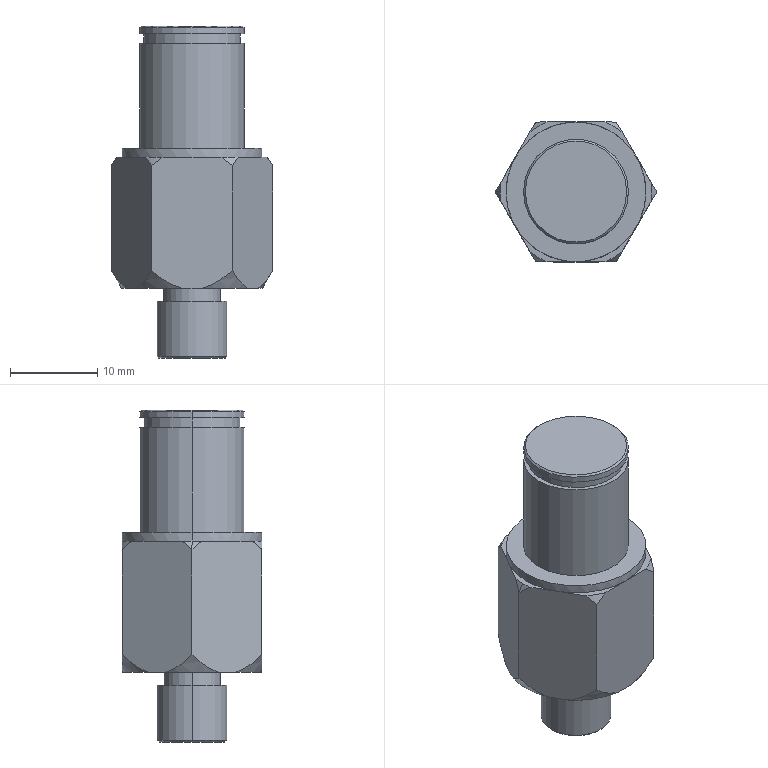Part | SolidWorks | features Cut 3, ICE 3, Chamfer 1, Extrusion 1, RevCut 1 | 1 solid | 49 faces | box 18.475 x 16 x 38 mm | volume 5453 mm3 | plane 19 | cone 18 | cylinder 12 | commonest cylinder face diameters 12 x4 6.5 x2 8 x2 11 x2 16 x2
STEP:
#1=CARTESIAN_POINT('',(-8.587,48.872,15.));
#2=VERTEX_POINT('',#1);
#3=CARTESIAN_POINT('',(-8.66,50.,15.));
#4=VERTEX_POINT('',#3);
#5=CARTESIAN_POINT('',(0.,50.,15.));
#6=DIRECTION('',(0.,0.,-1.));
#7=DIRECTION('',(-1.,0.,0.));
#8=AXIS2_PLACEMENT_3D('',#5,#6,#7);
#9=CIRCLE('',#8,8.66);
#10=EDGE_CURVE('',#2,#4,#9,.T.);
#11=ORIENTED_EDGE('',*,*,#10,.T.);
#12=CARTESIAN_POINT('',(-9.238,50.,14.));
#13=VERTEX_POINT('',#12);
#14=CARTESIAN_POINT('',(-8.66,50.,15.));
#15=DIRECTION('',(-0.5,0.,-0.866));
#16=VECTOR('',#15,1000.);
#17=LINE('',#14,#16);
#18=EDGE_CURVE('',#4,#13,#17,.T.);
#19=ORIENTED_EDGE('',*,*,#18,.T.);
#20=CARTESIAN_POINT('',(-9.238,50.,14.));
#21=CARTESIAN_POINT('',(-9.03,49.641,14.359));
#22=CARTESIAN_POINT('',(-8.815,49.268,14.697));
#23=CARTESIAN_POINT('',(-8.587,48.872,15.));
#24=B_SPLINE_CURVE_WITH_KNOTS('',3,(#20,#21,#22,#23),.UNSPECIFIED.,.F.,.F.,(4,4),(0.007442,0.009078),.UNSPECIFIED.);
#25=EDGE_CURVE('',#13,#2,#24,.T.);
#26=ORIENTED_EDGE('',*,*,#25,.T.);
#27=EDGE_LOOP('',(#11,#19,#26));
#28=FACE_OUTER_BOUND('',#27,.T.);
#29=CARTESIAN_POINT('',(0.,50.,15.));
#30=DIRECTION('',(0.,0.,-1.));
#31=DIRECTION('',(-1.,0.,0.));
#32=AXIS2_PLACEMENT_3D('',#29,#30,#31);
#33=CONICAL_SURFACE('',#32,8.66,0.5236);
#34=ADVANCED_FACE('',(#28),#33,.T.);
#35=CARTESIAN_POINT('',(8.083,50.,0.));
#36=VERTEX_POINT('',#35);
#37=CARTESIAN_POINT('',(7.506,47.,0.));
#38=VERTEX_POINT('',#37);
#39=CARTESIAN_POINT('',(0.,50.,0.));
#40=DIRECTION('',(0.,0.,-1.));
#41=DIRECTION('',(-1.,0.,0.));
#42=AXIS2_PLACEMENT_3D('',#39,#40,#41);
#43=CIRCLE('',#42,8.083);
#44=EDGE_CURVE('',#36,#38,#43,.T.);
#45=ORIENTED_EDGE('',*,*,#44,.F.);
#46=CARTESIAN_POINT('',(9.238,50.,2.));
#47=VERTEX_POINT('',#46);
#48=CARTESIAN_POINT('',(9.238,50.,2.));
#49=DIRECTION('',(0.5,0.,0.866));
#50=VECTOR('',#49,1000.);
#51=LINE('',#48,#50);
#52=EDGE_CURVE('',#36,#47,#51,.T.);
#53=ORIENTED_EDGE('',*,*,#52,.T.);
#54=CARTESIAN_POINT('',(9.238,50.,2.));
#55=CARTESIAN_POINT('',(8.982,49.558,1.558));
#56=CARTESIAN_POINT('',(8.714,49.094,1.146));
#57=CARTESIAN_POINT('',(8.136,48.093,0.4442));
#58=CARTESIAN_POINT('',(7.833,47.568,0.1622));
#59=CARTESIAN_POINT('',(7.506,47.,0.));
#60=B_SPLINE_CURVE_WITH_KNOTS('',3,(#54,#55,#56,#57,#58,#59),.UNSPECIFIED.,.F.,.F.,(4,2,4),(0.007563,0.009578,0.01159),.UNSPECIFIED.);
#61=EDGE_CURVE('',#47,#38,#60,.T.);
#62=ORIENTED_EDGE('',*,*,#61,.T.);
#63=EDGE_LOOP('',(#45,#53,#62));
#64=FACE_OUTER_BOUND('',#63,.T.);
#65=CARTESIAN_POINT('',(0.,50.,2.));
#66=DIRECTION('',(0.,0.,1.));
#67=DIRECTION('',(1.,0.,0.));
#68=AXIS2_PLACEMENT_3D('',#65,#66,#67);
#69=CONICAL_SURFACE('',#68,9.238,0.5236);
#70=ADVANCED_FACE('',(#64),#69,.T.);
#71=CARTESIAN_POINT('',(5.8,50.,30.));
#72=VERTEX_POINT('',#71);
#73=CARTESIAN_POINT('',(-5.8,50.,30.));
#74=VERTEX_POINT('',#73);
#75=CARTESIAN_POINT('',(0.,50.,30.));
#76=DIRECTION('',(0.,0.,1.));
#77=DIRECTION('',(1.,0.,0.));
#78=AXIS2_PLACEMENT_3D('',#75,#76,#77);
#79=CIRCLE('',#78,5.8);
#80=EDGE_CURVE('',#72,#74,#79,.T.);
#81=ORIENTED_EDGE('',*,*,#80,.F.);
#82=CARTESIAN_POINT('',(6.,50.,29.8));
#83=VERTEX_POINT('',#82);
#84=CARTESIAN_POINT('',(5.8,50.,30.));
#85=DIRECTION('',(0.7071,0.,-0.7071));
#86=VECTOR('',#85,1000.);
#87=LINE('',#84,#86);
#88=EDGE_CURVE('',#72,#83,#87,.T.);
#89=ORIENTED_EDGE('',*,*,#88,.T.);
#90=CARTESIAN_POINT('',(-6.,50.,29.8));
#91=VERTEX_POINT('',#90);
#92=CARTESIAN_POINT('',(0.,50.,29.8));
#93=DIRECTION('',(0.,0.,-1.));
#94=DIRECTION('',(1.,0.,0.));
#95=AXIS2_PLACEMENT_3D('',#92,#93,#94);
#96=CIRCLE('',#95,6.);
#97=EDGE_CURVE('',#91,#83,#96,.T.);
#98=ORIENTED_EDGE('',*,*,#97,.F.);
#99=CARTESIAN_POINT('',(-5.8,50.,30.));
#100=DIRECTION('',(-0.7071,0.,-0.7071));
#101=VECTOR('',#100,1000.);
#102=LINE('',#99,#101);
#103=EDGE_CURVE('',#74,#91,#102,.T.);
#104=ORIENTED_EDGE('',*,*,#103,.F.);
#105=EDGE_LOOP('',(#81,#89,#98,#104));
#106=FACE_OUTER_BOUND('',#105,.T.);
#107=CARTESIAN_POINT('',(0.,50.,30.));
#108=DIRECTION('',(0.,0.,-1.));
#109=DIRECTION('',(-1.,0.,0.));
#110=AXIS2_PLACEMENT_3D('',#107,#108,#109);
#111=CONICAL_SURFACE('',#110,5.8,0.7854);
#112=ADVANCED_FACE('',(#106),#111,.T.);
#113=CARTESIAN_POINT('',(-3.8,50.,-8.));
#114=VERTEX_POINT('',#113);
#115=CARTESIAN_POINT('',(3.8,50.,-8.));
#116=VERTEX_POINT('',#115);
#117=CARTESIAN_POINT('',(0.,50.,-8.));
#118=DIRECTION('',(0.,0.,-1.));
#119=DIRECTION('',(-1.,0.,0.));
#120=AXIS2_PLACEMENT_3D('',#117,#118,#119);
#121=CIRCLE('',#120,3.8);
#122=EDGE_CURVE('',#114,#116,#121,.T.);
#123=ORIENTED_EDGE('',*,*,#122,.F.);
#124=CARTESIAN_POINT('',(-4.,50.,-7.8));
#125=VERTEX_POINT('',#124);
#126=CARTESIAN_POINT('',(-3.8,50.,-8.));
#127=DIRECTION('',(-0.7071,0.,0.7071));
#128=VECTOR('',#127,1000.);
#129=LINE('',#126,#128);
#130=EDGE_CURVE('',#114,#125,#129,.T.);
#131=ORIENTED_EDGE('',*,*,#130,.T.);
#132=CARTESIAN_POINT('',(4.,50.,-7.8));
#133=VERTEX_POINT('',#132);
#134=CARTESIAN_POINT('',(0.,50.,-7.8));
#135=DIRECTION('',(0.,0.,1.));
#136=DIRECTION('',(-1.,0.,0.));
#137=AXIS2_PLACEMENT_3D('',#134,#135,#136);
#138=CIRCLE('',#137,4.);
#139=EDGE_CURVE('',#133,#125,#138,.T.);
#140=ORIENTED_EDGE('',*,*,#139,.F.);
#141=CARTESIAN_POINT('',(3.8,50.,-8.));
#142=DIRECTION('',(0.7071,0.,0.7071));
#143=VECTOR('',#142,1000.);
#144=LINE('',#141,#143);
#145=EDGE_CURVE('',#116,#133,#144,.T.);
#146=ORIENTED_EDGE('',*,*,#145,.F.);
#147=EDGE_LOOP('',(#123,#131,#140,#146));
#148=FACE_OUTER_BOUND('',#147,.T.);
#149=CARTESIAN_POINT('',(0.,50.,-8.));
#150=DIRECTION('',(0.,0.,1.));
#151=DIRECTION('',(1.,0.,0.));
#152=AXIS2_PLACEMENT_3D('',#149,#150,#151);
#153=CONICAL_SURFACE('',#152,3.8,0.7854);
#154=ADVANCED_FACE('',(#148),#153,.T.);
#155=CARTESIAN_POINT('',(-6.,50.,29.1));
#156=VERTEX_POINT('',#155);
#157=CARTESIAN_POINT('',(6.,50.,29.1));
#158=VERTEX_POINT('',#157);
#159=CARTESIAN_POINT('',(0.,50.,29.1));
#160=DIRECTION('',(0.,0.,-1.));
#161=DIRECTION('',(1.,0.,0.));
#162=AXIS2_PLACEMENT_3D('',#159,#160,#161);
#163=CIRCLE('',#162,6.);
#164=EDGE_CURVE('',#156,#158,#163,.T.);
#165=ORIENTED_EDGE('',*,*,#164,.F.);
#166=CARTESIAN_POINT('',(-6.,50.,16.));
#167=DIRECTION('',(0.,0.,1.));
#168=VECTOR('',#167,1000.);
#169=LINE('',#166,#168);
#170=EDGE_CURVE('',#156,#91,#169,.T.);
#171=ORIENTED_EDGE('',*,*,#170,.T.);
#172=ORIENTED_EDGE('',*,*,#97,.T.);
#173=CARTESIAN_POINT('',(6.,50.,16.));
#174=DIRECTION('',(0.,0.,1.));
#175=VECTOR('',#174,1000.);
#176=LINE('',#173,#175);
#177=EDGE_CURVE('',#158,#83,#176,.T.);
#178=ORIENTED_EDGE('',*,*,#177,.F.);
#179=EDGE_LOOP('',(#165,#171,#172,#178));
#180=FACE_OUTER_BOUND('',#179,.T.);
#181=CARTESIAN_POINT('',(0.,50.,16.));
#182=DIRECTION('',(0.,0.,1.));
#183=DIRECTION('',(1.,0.,0.));
#184=AXIS2_PLACEMENT_3D('',#181,#182,#183);
#185=CYLINDRICAL_SURFACE('',#184,6.);
#186=ADVANCED_FACE('',(#180),#185,.T.);
#187=CARTESIAN_POINT('',(5.5,50.,29.1));
#188=VERTEX_POINT('',#187);
#189=CARTESIAN_POINT('',(-5.5,50.,29.1));
#190=VERTEX_POINT('',#189);
#191=CARTESIAN_POINT('',(0.,50.,29.1));
#192=DIRECTION('',(0.,0.,1.));
#193=DIRECTION('',(1.,0.,0.));
#194=AXIS2_PLACEMENT_3D('',#191,#192,#193);
#195=CIRCLE('',#194,5.5);
#196=EDGE_CURVE('',#188,#190,#195,.T.);
#197=ORIENTED_EDGE('',*,*,#196,.F.);
#198=CARTESIAN_POINT('',(5.5,50.,28.));
#199=VERTEX_POINT('',#198);
#200=CARTESIAN_POINT('',(5.5,50.,29.1));
#201=DIRECTION('',(0.,0.,-1.));
#202=VECTOR('',#201,1000.);
#203=LINE('',#200,#202);
#204=EDGE_CURVE('',#188,#199,#203,.T.);
#205=ORIENTED_EDGE('',*,*,#204,.T.);
#206=CARTESIAN_POINT('',(-5.5,50.,28.));
#207=VERTEX_POINT('',#206);
#208=CARTESIAN_POINT('',(0.,50.,28.));
#209=DIRECTION('',(0.,0.,1.));
#210=DIRECTION('',(1.,0.,0.));
#211=AXIS2_PLACEMENT_3D('',#208,#209,#210);
#212=CIRCLE('',#211,5.5);
#213=EDGE_CURVE('',#199,#207,#212,.T.);
#214=ORIENTED_EDGE('',*,*,#213,.T.);
#215=CARTESIAN_POINT('',(-5.5,50.,29.1));
#216=DIRECTION('',(0.,0.,-1.));
#217=VECTOR('',#216,1000.);
#218=LINE('',#215,#217);
#219=EDGE_CURVE('',#190,#207,#218,.T.);
#220=ORIENTED_EDGE('',*,*,#219,.F.);
#221=EDGE_LOOP('',(#197,#205,#214,#220));
#222=FACE_OUTER_BOUND('',#221,.T.);
#223=CARTESIAN_POINT('',(0.,50.,29.1));
#224=DIRECTION('',(0.,0.,-1.));
#225=DIRECTION('',(-1.,0.,0.));
#226=AXIS2_PLACEMENT_3D('',#223,#224,#225);
#227=CYLINDRICAL_SURFACE('',#226,5.5);
#228=ADVANCED_FACE('',(#222),#227,.T.);
#229=ORIENTED_EDGE('',*,*,#139,.T.);
#230=CARTESIAN_POINT('',(-4.,50.,-1.5));
#231=VERTEX_POINT('',#230);
#232=CARTESIAN_POINT('',(-4.,50.,-8.));
#233=DIRECTION('',(0.,0.,1.));
#234=VECTOR('',#233,1000.);
#235=LINE('',#232,#234);
#236=EDGE_CURVE('',#125,#231,#235,.T.);
#237=ORIENTED_EDGE('',*,*,#236,.T.);
#238=CARTESIAN_POINT('',(4.,50.,-1.5));
#239=VERTEX_POINT('',#238);
#240=CARTESIAN_POINT('',(0.,50.,-1.5));
#241=DIRECTION('',(0.,0.,-1.));
#242=DIRECTION('',(-1.,0.,0.));
#243=AXIS2_PLACEMENT_3D('',#240,#241,#242);
#244=CIRCLE('',#243,4.);
#245=EDGE_CURVE('',#231,#239,#244,.T.);
#246=ORIENTED_EDGE('',*,*,#245,.T.);
#247=CARTESIAN_POINT('',(4.,50.,-8.));
#248=DIRECTION('',(0.,0.,1.));
#249=VECTOR('',#248,1000.);
#250=LINE('',#247,#249);
#251=EDGE_CURVE('',#133,#239,#250,.T.);
#252=ORIENTED_EDGE('',*,*,#251,.F.);
#253=EDGE_LOOP('',(#229,#237,#246,#252));
#254=FACE_OUTER_BOUND('',#253,.T.);
#255=CARTESIAN_POINT('',(0.,50.,-8.));
#256=DIRECTION('',(0.,0.,1.));
#257=DIRECTION('',(1.,0.,0.));
#258=AXIS2_PLACEMENT_3D('',#255,#256,#257);
#259=CYLINDRICAL_SURFACE('',#258,4.);
#260=ADVANCED_FACE('',(#254),#259,.T.);
#261=CARTESIAN_POINT('',(-3.25,50.,-1.5));
#262=VERTEX_POINT('',#261);
#263=CARTESIAN_POINT('',(3.25,50.,-1.5));
#264=VERTEX_POINT('',#263);
#265=CARTESIAN_POINT('',(0.,50.,-1.5));
#266=DIRECTION('',(0.,0.,-1.));
#267=DIRECTION('',(-1.,0.,0.));
#268=AXIS2_PLACEMENT_3D('',#265,#266,#267);
#269=CIRCLE('',#268,3.25);
#270=EDGE_CURVE('',#262,#264,#269,.T.);
#271=ORIENTED_EDGE('',*,*,#270,.F.);
#272=CARTESIAN_POINT('',(-3.25,50.,0.));
#273=VERTEX_POINT('',#272);
#274=CARTESIAN_POINT('',(-3.25,50.,-1.5));
#275=DIRECTION('',(0.,0.,1.));
#276=VECTOR('',#275,1000.);
#277=LINE('',#274,#276);
#278=EDGE_CURVE('',#262,#273,#277,.T.);
#279=ORIENTED_EDGE('',*,*,#278,.T.);
#280=CARTESIAN_POINT('',(3.25,50.,0.));
#281=VERTEX_POINT('',#280);
#282=CARTESIAN_POINT('',(0.,50.,0.));
#283=DIRECTION('',(0.,0.,-1.));
#284=DIRECTION('',(-1.,0.,0.));
#285=AXIS2_PLACEMENT_3D('',#282,#283,#284);
#286=CIRCLE('',#285,3.25);
#287=EDGE_CURVE('',#273,#281,#286,.T.);
#288=ORIENTED_EDGE('',*,*,#287,.T.);
#289=CARTESIAN_POINT('',(3.25,50.,-1.5));
#290=DIRECTION('',(0.,0.,1.));
#291=VECTOR('',#290,1000.);
#292=LINE('',#289,#291);
#293=EDGE_CURVE('',#264,#281,#292,.T.);
#294=ORIENTED_EDGE('',*,*,#293,.F.);
#295=EDGE_LOOP('',(#271,#279,#288,#294));
#296=FACE_OUTER_BOUND('',#295,.T.);
#297=CARTESIAN_POINT('',(0.,50.,-1.5));
#298=DIRECTION('',(0.,0.,1.));
#299=DIRECTION('',(1.,0.,0.));
#300=AXIS2_PLACEMENT_3D('',#297,#298,#299);
#301=CYLINDRICAL_SURFACE('',#300,3.25);
#302=ADVANCED_FACE('',(#296),#301,.T.);
#303=CARTESIAN_POINT('',(-8.,50.,16.));
#304=VERTEX_POINT('',#303);
#305=CARTESIAN_POINT('',(8.,50.,16.));
#306=VERTEX_POINT('',#305);
#307=CARTESIAN_POINT('',(0.,50.,16.));
#308=DIRECTION('',(0.,0.,-1.));
#309=DIRECTION('',(1.,0.,0.));
#310=AXIS2_PLACEMENT_3D('',#307,#308,#309);
#311=CIRCLE('',#310,8.);
#312=EDGE_CURVE('',#304,#306,#311,.T.);
#313=ORIENTED_EDGE('',*,*,#312,.T.);
#314=CARTESIAN_POINT('',(8.,50.,15.));
#315=VERTEX_POINT('',#314);
#316=CARTESIAN_POINT('',(8.,50.,30.));
#317=DIRECTION('',(0.,0.,-1.));
#318=VECTOR('',#317,1000.);
#319=LINE('',#316,#318);
#320=EDGE_CURVE('',#306,#315,#319,.T.);
#321=ORIENTED_EDGE('',*,*,#320,.T.);
#322=CARTESIAN_POINT('',(6.928,54.,15.));
#323=VERTEX_POINT('',#322);
#324=CARTESIAN_POINT('',(0.,50.,15.));
#325=DIRECTION('',(0.,0.,-1.));
#326=DIRECTION('',(-1.,0.,0.));
#327=AXIS2_PLACEMENT_3D('',#324,#325,#326);
#328=CIRCLE('',#327,8.);
#329=EDGE_CURVE('',#323,#315,#328,.T.);
#330=ORIENTED_EDGE('',*,*,#329,.F.);
#331=CARTESIAN_POINT('',(0.,58.,15.));
#332=VERTEX_POINT('',#331);
#333=CARTESIAN_POINT('',(0.,50.,15.));
#334=DIRECTION('',(0.,0.,-1.));
#335=DIRECTION('',(-1.,0.,0.));
#336=AXIS2_PLACEMENT_3D('',#333,#334,#335);
#337=CIRCLE('',#336,8.);
#338=EDGE_CURVE('',#332,#323,#337,.T.);
#339=ORIENTED_EDGE('',*,*,#338,.F.);
#340=CARTESIAN_POINT('',(-6.928,54.,15.));
#341=VERTEX_POINT('',#340);
#342=CARTESIAN_POINT('',(0.,50.,15.));
#343=DIRECTION('',(0.,0.,-1.));
#344=DIRECTION('',(-1.,0.,0.));
#345=AXIS2_PLACEMENT_3D('',#342,#343,#344);
#346=CIRCLE('',#345,8.);
#347=EDGE_CURVE('',#341,#332,#346,.T.);
#348=ORIENTED_EDGE('',*,*,#347,.F.);
#349=CARTESIAN_POINT('',(-8.,50.,15.));
#350=VERTEX_POINT('',#349);
#351=CARTESIAN_POINT('',(0.,50.,15.));
#352=DIRECTION('',(0.,0.,-1.));
#353=DIRECTION('',(-1.,0.,0.));
#354=AXIS2_PLACEMENT_3D('',#351,#352,#353);
#355=CIRCLE('',#354,8.);
#356=EDGE_CURVE('',#350,#341,#355,.T.);
#357=ORIENTED_EDGE('',*,*,#356,.F.);
#358=CARTESIAN_POINT('',(-8.,50.,30.));
#359=DIRECTION('',(0.,0.,-1.));
#360=VECTOR('',#359,1000.);
#361=LINE('',#358,#360);
#362=EDGE_CURVE('',#304,#350,#361,.T.);
#363=ORIENTED_EDGE('',*,*,#362,.F.);
#364=EDGE_LOOP('',(#313,#321,#330,#339,#348,#357,#363));
#365=FACE_OUTER_BOUND('',#364,.T.);
#366=CARTESIAN_POINT('',(0.,50.,30.));
#367=DIRECTION('',(0.,0.,-1.));
#368=DIRECTION('',(-1.,0.,0.));
#369=AXIS2_PLACEMENT_3D('',#366,#367,#368);
#370=CYLINDRICAL_SURFACE('',#369,8.);
#371=ADVANCED_FACE('',(#365),#370,.T.);
#372=CARTESIAN_POINT('',(6.,50.,16.));
#373=VERTEX_POINT('',#372);
#374=CARTESIAN_POINT('',(-6.,50.,16.));
#375=VERTEX_POINT('',#374);
#376=CARTESIAN_POINT('',(0.,50.,16.));
#377=DIRECTION('',(0.,0.,1.));
#378=DIRECTION('',(1.,0.,0.));
#379=AXIS2_PLACEMENT_3D('',#376,#377,#378);
#380=CIRCLE('',#379,6.);
#381=EDGE_CURVE('',#373,#375,#380,.T.);
#382=ORIENTED_EDGE('',*,*,#381,.T.);
#383=CARTESIAN_POINT('',(-6.,50.,28.));
#384=VERTEX_POINT('',#383);
#385=CARTESIAN_POINT('',(-6.,50.,16.));
#386=DIRECTION('',(0.,0.,1.));
#387=VECTOR('',#386,1000.);
#388=LINE('',#385,#387);
#389=EDGE_CURVE('',#375,#384,#388,.T.);
#390=ORIENTED_EDGE('',*,*,#389,.T.);
#391=CARTESIAN_POINT('',(6.,50.,28.));
#392=VERTEX_POINT('',#391);
#393=CARTESIAN_POINT('',(0.,50.,28.));
#394=DIRECTION('',(0.,0.,-1.));
#395=DIRECTION('',(1.,0.,0.));
#396=AXIS2_PLACEMENT_3D('',#393,#394,#395);
#397=CIRCLE('',#396,6.);
#398=EDGE_CURVE('',#384,#392,#397,.T.);
#399=ORIENTED_EDGE('',*,*,#398,.T.);
#400=CARTESIAN_POINT('',(6.,50.,16.));
#401=DIRECTION('',(0.,0.,1.));
#402=VECTOR('',#401,1000.);
#403=LINE('',#400,#402);
#404=EDGE_CURVE('',#373,#392,#403,.T.);
#405=ORIENTED_EDGE('',*,*,#404,.F.);
#406=EDGE_LOOP('',(#382,#390,#399,#405));
#407=FACE_OUTER_BOUND('',#406,.T.);
#408=CARTESIAN_POINT('',(0.,50.,16.));
#409=DIRECTION('',(0.,0.,1.));
#410=DIRECTION('',(1.,0.,0.));
#411=AXIS2_PLACEMENT_3D('',#408,#409,#410);
#412=CYLINDRICAL_SURFACE('',#411,6.);
#413=ADVANCED_FACE('',(#407),#412,.T.);
#414=ORIENTED_EDGE('',*,*,#389,.F.);
#415=CARTESIAN_POINT('',(0.,50.,16.));
#416=DIRECTION('',(0.,0.,1.));
#417=DIRECTION('',(1.,0.,0.));
#418=AXIS2_PLACEMENT_3D('',#415,#416,#417);
#419=CIRCLE('',#418,6.);
#420=EDGE_CURVE('',#375,#373,#419,.T.);
#421=ORIENTED_EDGE('',*,*,#420,.T.);
#422=ORIENTED_EDGE('',*,*,#404,.T.);
#423=CARTESIAN_POINT('',(0.,50.,28.));
#424=DIRECTION('',(0.,0.,-1.));
#425=DIRECTION('',(1.,0.,0.));
#426=AXIS2_PLACEMENT_3D('',#423,#424,#425);
#427=CIRCLE('',#426,6.);
#428=EDGE_CURVE('',#392,#384,#427,.T.);
#429=ORIENTED_EDGE('',*,*,#428,.T.);
#430=EDGE_LOOP('',(#414,#421,#422,#429));
#431=FACE_OUTER_BOUND('',#430,.T.);
#432=CARTESIAN_POINT('',(0.,50.,16.));
#433=DIRECTION('',(0.,0.,1.));
#434=DIRECTION('',(1.,0.,0.));
#435=AXIS2_PLACEMENT_3D('',#432,#433,#434);
#436=CYLINDRICAL_SURFACE('',#435,6.);
#437=ADVANCED_FACE('',(#431),#436,.T.);
#438=ORIENTED_EDGE('',*,*,#320,.F.);
#439=CARTESIAN_POINT('',(0.,50.,16.));
#440=DIRECTION('',(0.,0.,-1.));
#441=DIRECTION('',(1.,0.,0.));
#442=AXIS2_PLACEMENT_3D('',#439,#440,#441);
#443=CIRCLE('',#442,8.);
#444=EDGE_CURVE('',#306,#304,#443,.T.);
#445=ORIENTED_EDGE('',*,*,#444,.T.);
#446=ORIENTED_EDGE('',*,*,#362,.T.);
#447=CARTESIAN_POINT('',(-6.928,46.,15.));
#448=VERTEX_POINT('',#447);
#449=CARTESIAN_POINT('',(0.,50.,15.));
#450=DIRECTION('',(0.,0.,-1.));
#451=DIRECTION('',(-1.,0.,0.));
#452=AXIS2_PLACEMENT_3D('',#449,#450,#451);
#453=CIRCLE('',#452,8.);
#454=EDGE_CURVE('',#448,#350,#453,.T.);
#455=ORIENTED_EDGE('',*,*,#454,.F.);
#456=CARTESIAN_POINT('',(0.,42.,15.));
#457=VERTEX_POINT('',#456);
#458=CARTESIAN_POINT('',(0.,50.,15.));
#459=DIRECTION('',(0.,0.,-1.));
#460=DIRECTION('',(-1.,0.,0.));
#461=AXIS2_PLACEMENT_3D('',#458,#459,#460);
#462=CIRCLE('',#461,8.);
#463=EDGE_CURVE('',#457,#448,#462,.T.);
#464=ORIENTED_EDGE('',*,*,#463,.F.);
#465=CARTESIAN_POINT('',(6.928,46.,15.));
#466=VERTEX_POINT('',#465);
#467=CARTESIAN_POINT('',(0.,50.,15.));
#468=DIRECTION('',(0.,0.,-1.));
#469=DIRECTION('',(-1.,0.,0.));
#470=AXIS2_PLACEMENT_3D('',#467,#468,#469);
#471=CIRCLE('',#470,8.);
#472=EDGE_CURVE('',#466,#457,#471,.T.);
#473=ORIENTED_EDGE('',*,*,#472,.F.);
#474=CARTESIAN_POINT('',(0.,50.,15.));
#475=DIRECTION('',(0.,0.,-1.));
#476=DIRECTION('',(-1.,0.,0.));
#477=AXIS2_PLACEMENT_3D('',#474,#475,#476);
#478=CIRCLE('',#477,8.);
#479=EDGE_CURVE('',#315,#466,#478,.T.);
#480=ORIENTED_EDGE('',*,*,#479,.F.);
#481=EDGE_LOOP('',(#438,#445,#446,#455,#464,#473,#480));
#482=FACE_OUTER_BOUND('',#481,.T.);
#483=CARTESIAN_POINT('',(0.,50.,30.));
#484=DIRECTION('',(0.,0.,-1.));
#485=DIRECTION('',(-1.,0.,0.));
#486=AXIS2_PLACEMENT_3D('',#483,#484,#485);
#487=CYLINDRICAL_SURFACE('',#486,8.);
#488=ADVANCED_FACE('',(#482),#487,.T.);
#489=CARTESIAN_POINT('',(6.351,45.,0.));
#490=VERTEX_POINT('',#489);
#491=CARTESIAN_POINT('',(9.238,50.,0.));
#492=DIRECTION('',(-0.5,-0.866,0.));
#493=VECTOR('',#492,1000.);
#494=LINE('',#491,#493);
#495=EDGE_CURVE('',#38,#490,#494,.T.);
#496=ORIENTED_EDGE('',*,*,#495,.T.);
#497=CARTESIAN_POINT('',(1.155,42.,0.));
#498=VERTEX_POINT('',#497);
#499=CARTESIAN_POINT('',(0.,50.,0.));
#500=DIRECTION('',(0.,0.,-1.));
#501=DIRECTION('',(-1.,0.,0.));
#502=AXIS2_PLACEMENT_3D('',#499,#500,#501);
#503=CIRCLE('',#502,8.083);
#504=EDGE_CURVE('',#490,#498,#503,.T.);
#505=ORIENTED_EDGE('',*,*,#504,.T.);
#506=CARTESIAN_POINT('',(-1.155,42.,0.));
#507=VERTEX_POINT('',#506);
#508=CARTESIAN_POINT('',(4.619,42.,0.));
#509=DIRECTION('',(-1.,0.,0.));
#510=VECTOR('',#509,1000.);
#511=LINE('',#508,#510);
#512=EDGE_CURVE('',#498,#507,#511,.T.);
#513=ORIENTED_EDGE('',*,*,#512,.T.);
#514=CARTESIAN_POINT('',(-6.351,45.,0.));
#515=VERTEX_POINT('',#514);
#516=CARTESIAN_POINT('',(0.,50.,0.));
#517=DIRECTION('',(0.,0.,-1.));
#518=DIRECTION('',(-1.,0.,0.));
#519=AXIS2_PLACEMENT_3D('',#516,#517,#518);
#520=CIRCLE('',#519,8.083);
#521=EDGE_CURVE('',#507,#515,#520,.T.);
#522=ORIENTED_EDGE('',*,*,#521,.T.);
#523=CARTESIAN_POINT('',(-7.506,47.,0.));
#524=VERTEX_POINT('',#523);
#525=CARTESIAN_POINT('',(-4.619,42.,0.));
#526=DIRECTION('',(-0.5,0.866,0.));
#527=VECTOR('',#526,1000.);
#528=LINE('',#525,#527);
#529=EDGE_CURVE('',#515,#524,#528,.T.);
#530=ORIENTED_EDGE('',*,*,#529,.T.);
#531=CARTESIAN_POINT('',(-7.506,53.,0.));
#532=VERTEX_POINT('',#531);
#533=CARTESIAN_POINT('',(0.,50.,0.));
#534=DIRECTION('',(0.,0.,-1.));
#535=DIRECTION('',(-1.,0.,0.));
#536=AXIS2_PLACEMENT_3D('',#533,#534,#535);
#537=CIRCLE('',#536,8.083);
#538=EDGE_CURVE('',#524,#532,#537,.T.);
#539=ORIENTED_EDGE('',*,*,#538,.T.);
#540=CARTESIAN_POINT('',(-6.351,55.,0.));
#541=VERTEX_POINT('',#540);
#542=CARTESIAN_POINT('',(-9.238,50.,0.));
#543=DIRECTION('',(0.5,0.866,0.));
#544=VECTOR('',#543,1000.);
#545=LINE('',#542,#544);
#546=EDGE_CURVE('',#532,#541,#545,.T.);
#547=ORIENTED_EDGE('',*,*,#546,.T.);
#548=CARTESIAN_POINT('',(-1.155,58.,0.));
#549=VERTEX_POINT('',#548);
#550=CARTESIAN_POINT('',(0.,50.,0.));
#551=DIRECTION('',(0.,0.,-1.));
#552=DIRECTION('',(-1.,0.,0.));
#553=AXIS2_PLACEMENT_3D('',#550,#551,#552);
#554=CIRCLE('',#553,8.083);
#555=EDGE_CURVE('',#541,#549,#554,.T.);
#556=ORIENTED_EDGE('',*,*,#555,.T.);
#557=CARTESIAN_POINT('',(1.155,58.,0.));
#558=VERTEX_POINT('',#557);
#559=CARTESIAN_POINT('',(-4.619,58.,0.));
#560=DIRECTION('',(1.,0.,0.));
#561=VECTOR('',#560,1000.);
#562=LINE('',#559,#561);
#563=EDGE_CURVE('',#549,#558,#562,.T.);
#564=ORIENTED_EDGE('',*,*,#563,.T.);
#565=CARTESIAN_POINT('',(6.351,55.,0.));
#566=VERTEX_POINT('',#565);
#567=CARTESIAN_POINT('',(0.,50.,0.));
#568=DIRECTION('',(0.,0.,-1.));
#569=DIRECTION('',(-1.,0.,0.));
#570=AXIS2_PLACEMENT_3D('',#567,#568,#569);
#571=CIRCLE('',#570,8.083);
#572=EDGE_CURVE('',#558,#566,#571,.T.);
#573=ORIENTED_EDGE('',*,*,#572,.T.);
#574=CARTESIAN_POINT('',(7.506,53.,0.));
#575=VERTEX_POINT('',#574);
#576=CARTESIAN_POINT('',(4.619,58.,0.));
#577=DIRECTION('',(0.5,-0.866,0.));
#578=VECTOR('',#577,1000.);
#579=LINE('',#576,#578);
#580=EDGE_CURVE('',#566,#575,#579,.T.);
#581=ORIENTED_EDGE('',*,*,#580,.T.);
#582=CARTESIAN_POINT('',(0.,50.,0.));
#583=DIRECTION('',(0.,0.,-1.));
#584=DIRECTION('',(-1.,0.,0.));
#585=AXIS2_PLACEMENT_3D('',#582,#583,#584);
#586=CIRCLE('',#585,8.083);
#587=EDGE_CURVE('',#575,#36,#586,.T.);
#588=ORIENTED_EDGE('',*,*,#587,.T.);
#589=ORIENTED_EDGE('',*,*,#44,.T.);
#590=EDGE_LOOP('',(#496,#505,#513,#522,#530,#539,#547,#556,#564,#573,#581,#588,#589));
#591=FACE_OUTER_BOUND('',#590,.T.);
#592=CARTESIAN_POINT('',(0.,50.,0.));
#593=DIRECTION('',(0.,0.,-1.));
#594=DIRECTION('',(-1.,0.,0.));
#595=AXIS2_PLACEMENT_3D('',#592,#593,#594);
#596=CIRCLE('',#595,3.25);
#597=EDGE_CURVE('',#281,#273,#596,.T.);
#598=ORIENTED_EDGE('',*,*,#597,.F.);
#599=ORIENTED_EDGE('',*,*,#287,.F.);
#600=EDGE_LOOP('',(#598,#599));
#601=FACE_BOUND('',#600,.T.);
#602=CARTESIAN_POINT('',(0.,50.,0.));
#603=DIRECTION('',(0.,0.,1.));
#604=DIRECTION('',(1.,0.,0.));
#605=AXIS2_PLACEMENT_3D('',#602,#603,#604);
#606=PLANE('',#605);
#607=ADVANCED_FACE('',(#591,#601),#606,.F.);
#608=CARTESIAN_POINT('',(-4.619,42.,14.));
#609=VERTEX_POINT('',#608);
#610=CARTESIAN_POINT('',(-3.317,42.,15.));
#611=VERTEX_POINT('',#610);
#612=CARTESIAN_POINT('',(-4.619,42.,14.));
#613=CARTESIAN_POINT('',(-4.204,42.,14.359));
#614=CARTESIAN_POINT('',(-3.773,42.,14.697));
#615=CARTESIAN_POINT('',(-3.317,42.,15.));
#616=B_SPLINE_CURVE_WITH_KNOTS('',3,(#612,#613,#614,#615),.UNSPECIFIED.,.F.,.F.,(4,4),(0.007442,0.009078),.UNSPECIFIED.);
#617=EDGE_CURVE('',#609,#611,#616,.T.);
#618=ORIENTED_EDGE('',*,*,#617,.F.);
#619=CARTESIAN_POINT('',(-4.619,42.,2.));
#620=VERTEX_POINT('',#619);
#621=CARTESIAN_POINT('',(-4.619,42.,15.));
#622=DIRECTION('',(0.,0.,-1.));
#623=VECTOR('',#622,1000.);
#624=LINE('',#621,#623);
#625=EDGE_CURVE('',#609,#620,#624,.T.);
#626=ORIENTED_EDGE('',*,*,#625,.T.);
#627=CARTESIAN_POINT('',(-1.155,42.,0.));
#628=CARTESIAN_POINT('',(-1.482,42.,0.08107));
#629=CARTESIAN_POINT('',(-1.8,42.,0.1933));
#630=CARTESIAN_POINT('',(-2.419,42.,0.4666));
#631=CARTESIAN_POINT('',(-2.718,42.,0.627));
#632=CARTESIAN_POINT('',(-3.578,42.,1.151));
#633=CARTESIAN_POINT('',(-4.11,42.,1.559));
#634=CARTESIAN_POINT('',(-4.619,42.,2.));
#635=B_SPLINE_CURVE_WITH_KNOTS('',3,(#627,#628,#629,#630,#631,#632,#633,#634),.UNSPECIFIED.,.F.,.F.,(4,2,2,4),(0.01391,0.01491,0.01592,0.01793),.UNSPECIFIED.);
#636=EDGE_CURVE('',#507,#620,#635,.T.);
#637=ORIENTED_EDGE('',*,*,#636,.F.);
#638=ORIENTED_EDGE('',*,*,#512,.F.);
#639=CARTESIAN_POINT('',(4.619,42.,2.));
#640=VERTEX_POINT('',#639);
#641=CARTESIAN_POINT('',(4.619,42.,2.));
#642=CARTESIAN_POINT('',(4.109,42.,1.558));
#643=CARTESIAN_POINT('',(3.572,42.,1.146));
#644=CARTESIAN_POINT('',(2.416,42.,0.4442));
#645=CARTESIAN_POINT('',(1.81,42.,0.1622));
#646=CARTESIAN_POINT('',(1.155,42.,0.));
#647=B_SPLINE_CURVE_WITH_KNOTS('',3,(#641,#642,#643,#644,#645,#646),.UNSPECIFIED.,.F.,.F.,(4,2,4),(0.007563,0.009578,0.01159),.UNSPECIFIED.);
#648=EDGE_CURVE('',#640,#498,#647,.T.);
#649=ORIENTED_EDGE('',*,*,#648,.F.);
#650=CARTESIAN_POINT('',(4.619,42.,14.));
#651=VERTEX_POINT('',#650);
#652=CARTESIAN_POINT('',(4.619,42.,15.));
#653=DIRECTION('',(0.,0.,-1.));
#654=VECTOR('',#653,1000.);
#655=LINE('',#652,#654);
#656=EDGE_CURVE('',#651,#640,#655,.T.);
#657=ORIENTED_EDGE('',*,*,#656,.F.);
#658=CARTESIAN_POINT('',(3.317,42.,15.));
#659=VERTEX_POINT('',#658);
#660=CARTESIAN_POINT('',(3.317,42.,15.));
#661=CARTESIAN_POINT('',(3.772,42.,14.698));
#662=CARTESIAN_POINT('',(4.203,42.,14.36));
#663=CARTESIAN_POINT('',(4.619,42.,14.));
#664=B_SPLINE_CURVE_WITH_KNOTS('',3,(#660,#661,#662,#663),.UNSPECIFIED.,.F.,.F.,(4,4),(0.01616,0.0178),.UNSPECIFIED.);
#665=EDGE_CURVE('',#659,#651,#664,.T.);
#666=ORIENTED_EDGE('',*,*,#665,.F.);
#667=CARTESIAN_POINT('',(4.619,42.,15.));
#668=DIRECTION('',(-1.,0.,0.));
#669=VECTOR('',#668,1000.);
#670=LINE('',#667,#669);
#671=EDGE_CURVE('',#659,#457,#670,.T.);
#672=ORIENTED_EDGE('',*,*,#671,.T.);
#673=CARTESIAN_POINT('',(4.619,42.,15.));
#674=DIRECTION('',(-1.,0.,0.));
#675=VECTOR('',#674,1000.);
#676=LINE('',#673,#675);
#677=EDGE_CURVE('',#457,#611,#676,.T.);
#678=ORIENTED_EDGE('',*,*,#677,.T.);
#679=EDGE_LOOP('',(#618,#626,#637,#638,#649,#657,#666,#672,#678));
#680=FACE_OUTER_BOUND('',#679,.T.);
#681=CARTESIAN_POINT('',(4.619,42.,15.));
#682=DIRECTION('',(0.,-1.,0.));
#683=DIRECTION('',(0.,0.,-1.));
#684=AXIS2_PLACEMENT_3D('',#681,#682,#683);
#685=PLANE('',#684);
#686=ADVANCED_FACE('',(#680),#685,.T.);
#687=ORIENTED_EDGE('',*,*,#25,.F.);
#688=CARTESIAN_POINT('',(-9.238,50.,2.));
#689=VERTEX_POINT('',#688);
#690=CARTESIAN_POINT('',(-9.238,50.,15.));
#691=DIRECTION('',(0.,0.,-1.));
#692=VECTOR('',#691,1000.);
#693=LINE('',#690,#692);
#694=EDGE_CURVE('',#13,#689,#693,.T.);
#695=ORIENTED_EDGE('',*,*,#694,.T.);
#696=CARTESIAN_POINT('',(-7.506,47.,0.));
#697=CARTESIAN_POINT('',(-7.669,47.284,0.08107));
#698=CARTESIAN_POINT('',(-7.828,47.559,0.1933));
#699=CARTESIAN_POINT('',(-8.138,48.095,0.4666));
#700=CARTESIAN_POINT('',(-8.287,48.354,0.627));
#701=CARTESIAN_POINT('',(-8.717,49.099,1.151));
#702=CARTESIAN_POINT('',(-8.983,49.559,1.559));
#703=CARTESIAN_POINT('',(-9.238,50.,2.));
#704=B_SPLINE_CURVE_WITH_KNOTS('',3,(#696,#697,#698,#699,#700,#701,#702,#703),.UNSPECIFIED.,.F.,.F.,(4,2,2,4),(0.01391,0.01491,0.01592,0.01793),.UNSPECIFIED.);
#705=EDGE_CURVE('',#524,#689,#704,.T.);
#706=ORIENTED_EDGE('',*,*,#705,.F.);
#707=ORIENTED_EDGE('',*,*,#529,.F.);
#708=CARTESIAN_POINT('',(-4.619,42.,2.));
#709=CARTESIAN_POINT('',(-4.874,42.442,1.558));
#710=CARTESIAN_POINT('',(-5.142,42.906,1.146));
#711=CARTESIAN_POINT('',(-5.72,43.907,0.4442));
#712=CARTESIAN_POINT('',(-6.023,44.432,0.1622));
#713=CARTESIAN_POINT('',(-6.351,45.,0.));
#714=B_SPLINE_CURVE_WITH_KNOTS('',3,(#708,#709,#710,#711,#712,#713),.UNSPECIFIED.,.F.,.F.,(4,2,4),(0.007563,0.009578,0.01159),.UNSPECIFIED.);
#715=EDGE_CURVE('',#620,#515,#714,.T.);
#716=ORIENTED_EDGE('',*,*,#715,.F.);
#717=ORIENTED_EDGE('',*,*,#625,.F.);
#718=CARTESIAN_POINT('',(-5.27,43.128,15.));
#719=VERTEX_POINT('',#718);
#720=CARTESIAN_POINT('',(-5.27,43.128,15.));
#721=CARTESIAN_POINT('',(-5.042,42.734,14.698));
#722=CARTESIAN_POINT('',(-4.827,42.36,14.36));
#723=CARTESIAN_POINT('',(-4.619,42.,14.));
#724=B_SPLINE_CURVE_WITH_KNOTS('',3,(#720,#721,#722,#723),.UNSPECIFIED.,.F.,.F.,(4,4),(0.01616,0.0178),.UNSPECIFIED.);
#725=EDGE_CURVE('',#719,#609,#724,.T.);
#726=ORIENTED_EDGE('',*,*,#725,.F.);
#727=CARTESIAN_POINT('',(-4.619,42.,15.));
#728=DIRECTION('',(-0.5,0.866,0.));
#729=VECTOR('',#728,1000.);
#730=LINE('',#727,#729);
#731=EDGE_CURVE('',#719,#448,#730,.T.);
#732=ORIENTED_EDGE('',*,*,#731,.T.);
#733=CARTESIAN_POINT('',(-4.619,42.,15.));
#734=DIRECTION('',(0.5,-0.866,0.));
#735=VECTOR('',#734,1000.);
#736=LINE('',#733,#735);
#737=EDGE_CURVE('',#2,#448,#736,.T.);
#738=ORIENTED_EDGE('',*,*,#737,.F.);
#739=EDGE_LOOP('',(#687,#695,#706,#707,#716,#717,#726,#732,#738));
#740=FACE_OUTER_BOUND('',#739,.T.);
#741=CARTESIAN_POINT('',(-4.619,42.,15.));
#742=DIRECTION('',(-0.866,-0.5,0.));
#743=DIRECTION('',(0.5,-0.866,0.));
#744=AXIS2_PLACEMENT_3D('',#741,#742,#743);
#745=PLANE('',#744);
#746=ADVANCED_FACE('',(#740),#745,.T.);
#747=CARTESIAN_POINT('',(-4.619,58.,14.));
#748=VERTEX_POINT('',#747);
#749=CARTESIAN_POINT('',(-5.27,56.872,15.));
#750=VERTEX_POINT('',#749);
#751=CARTESIAN_POINT('',(-4.619,58.,14.));
#752=CARTESIAN_POINT('',(-4.826,57.641,14.359));
#753=CARTESIAN_POINT('',(-5.042,57.268,14.697));
#754=CARTESIAN_POINT('',(-5.27,56.872,15.));
#755=B_SPLINE_CURVE_WITH_KNOTS('',3,(#751,#752,#753,#754),.UNSPECIFIED.,.F.,.F.,(4,4),(0.007442,0.009078),.UNSPECIFIED.);
#756=EDGE_CURVE('',#748,#750,#755,.T.);
#757=ORIENTED_EDGE('',*,*,#756,.F.);
#758=CARTESIAN_POINT('',(-4.619,58.,2.));
#759=VERTEX_POINT('',#758);
#760=CARTESIAN_POINT('',(-4.619,58.,15.));
#761=DIRECTION('',(0.,0.,-1.));
#762=VECTOR('',#761,1000.);
#763=LINE('',#760,#762);
#764=EDGE_CURVE('',#748,#759,#763,.T.);
#765=ORIENTED_EDGE('',*,*,#764,.T.);
#766=CARTESIAN_POINT('',(-6.351,55.,0.));
#767=CARTESIAN_POINT('',(-6.187,55.284,0.08107));
#768=CARTESIAN_POINT('',(-6.028,55.559,0.1933));
#769=CARTESIAN_POINT('',(-5.719,56.095,0.4666));
#770=CARTESIAN_POINT('',(-5.569,56.354,0.627));
#771=CARTESIAN_POINT('',(-5.139,57.099,1.151));
#772=CARTESIAN_POINT('',(-4.873,57.559,1.559));
#773=CARTESIAN_POINT('',(-4.619,58.,2.));
#774=B_SPLINE_CURVE_WITH_KNOTS('',3,(#766,#767,#768,#769,#770,#771,#772,#773),.UNSPECIFIED.,.F.,.F.,(4,2,2,4),(0.01391,0.01491,0.01592,0.01793),.UNSPECIFIED.);
#775=EDGE_CURVE('',#541,#759,#774,.T.);
#776=ORIENTED_EDGE('',*,*,#775,.F.);
#777=ORIENTED_EDGE('',*,*,#546,.F.);
#778=CARTESIAN_POINT('',(-9.238,50.,2.));
#779=CARTESIAN_POINT('',(-8.982,50.442,1.558));
#780=CARTESIAN_POINT('',(-8.714,50.906,1.146));
#781=CARTESIAN_POINT('',(-8.136,51.907,0.4442));
#782=CARTESIAN_POINT('',(-7.833,52.432,0.1622));
#783=CARTESIAN_POINT('',(-7.506,53.,0.));
#784=B_SPLINE_CURVE_WITH_KNOTS('',3,(#778,#779,#780,#781,#782,#783),.UNSPECIFIED.,.F.,.F.,(4,2,4),(0.007563,0.009578,0.01159),.UNSPECIFIED.);
#785=EDGE_CURVE('',#689,#532,#784,.T.);
#786=ORIENTED_EDGE('',*,*,#785,.F.);
#787=ORIENTED_EDGE('',*,*,#694,.F.);
#788=CARTESIAN_POINT('',(-8.587,51.128,15.));
#789=VERTEX_POINT('',#788);
#790=CARTESIAN_POINT('',(-8.587,51.128,15.));
#791=CARTESIAN_POINT('',(-8.814,50.734,14.698));
#792=CARTESIAN_POINT('',(-9.03,50.36,14.36));
#793=CARTESIAN_POINT('',(-9.238,50.,14.));
#794=B_SPLINE_CURVE_WITH_KNOTS('',3,(#790,#791,#792,#793),.UNSPECIFIED.,.F.,.F.,(4,4),(0.01616,0.0178),.UNSPECIFIED.);
#795=EDGE_CURVE('',#789,#13,#794,.T.);
#796=ORIENTED_EDGE('',*,*,#795,.F.);
#797=CARTESIAN_POINT('',(-9.238,50.,15.));
#798=DIRECTION('',(0.5,0.866,0.));
#799=VECTOR('',#798,1000.);
#800=LINE('',#797,#799);
#801=EDGE_CURVE('',#789,#341,#800,.T.);
#802=ORIENTED_EDGE('',*,*,#801,.T.);
#803=CARTESIAN_POINT('',(-9.238,50.,15.));
#804=DIRECTION('',(-0.5,-0.866,0.));
#805=VECTOR('',#804,1000.);
#806=LINE('',#803,#805);
#807=EDGE_CURVE('',#750,#341,#806,.T.);
#808=ORIENTED_EDGE('',*,*,#807,.F.);
#809=EDGE_LOOP('',(#757,#765,#776,#777,#786,#787,#796,#802,#808));
#810=FACE_OUTER_BOUND('',#809,.T.);
#811=CARTESIAN_POINT('',(-9.238,50.,15.));
#812=DIRECTION('',(-0.866,0.5,0.));
#813=DIRECTION('',(-0.5,-0.866,0.));
#814=AXIS2_PLACEMENT_3D('',#811,#812,#813);
#815=PLANE('',#814);
#816=ADVANCED_FACE('',(#810),#815,.T.);
#817=CARTESIAN_POINT('',(4.619,58.,14.));
#818=VERTEX_POINT('',#817);
#819=CARTESIAN_POINT('',(3.317,58.,15.));
#820=VERTEX_POINT('',#819);
#821=CARTESIAN_POINT('',(4.619,58.,14.));
#822=CARTESIAN_POINT('',(4.204,58.,14.359));
#823=CARTESIAN_POINT('',(3.773,58.,14.697));
#824=CARTESIAN_POINT('',(3.317,58.,15.));
#825=B_SPLINE_CURVE_WITH_KNOTS('',3,(#821,#822,#823,#824),.UNSPECIFIED.,.F.,.F.,(4,4),(0.007442,0.009078),.UNSPECIFIED.);
#826=EDGE_CURVE('',#818,#820,#825,.T.);
#827=ORIENTED_EDGE('',*,*,#826,.F.);
#828=CARTESIAN_POINT('',(4.619,58.,2.));
#829=VERTEX_POINT('',#828);
#830=CARTESIAN_POINT('',(4.619,58.,15.));
#831=DIRECTION('',(0.,0.,-1.));
#832=VECTOR('',#831,1000.);
#833=LINE('',#830,#832);
#834=EDGE_CURVE('',#818,#829,#833,.T.);
#835=ORIENTED_EDGE('',*,*,#834,.T.);
#836=CARTESIAN_POINT('',(1.155,58.,0.));
#837=CARTESIAN_POINT('',(1.482,58.,0.08107));
#838=CARTESIAN_POINT('',(1.8,58.,0.1933));
#839=CARTESIAN_POINT('',(2.419,58.,0.4666));
#840=CARTESIAN_POINT('',(2.718,58.,0.627));
#841=CARTESIAN_POINT('',(3.578,58.,1.151));
#842=CARTESIAN_POINT('',(4.11,58.,1.559));
#843=CARTESIAN_POINT('',(4.619,58.,2.));
#844=B_SPLINE_CURVE_WITH_KNOTS('',3,(#836,#837,#838,#839,#840,#841,#842,#843),.UNSPECIFIED.,.F.,.F.,(4,2,2,4),(0.01391,0.01491,0.01592,0.01793),.UNSPECIFIED.);
#845=EDGE_CURVE('',#558,#829,#844,.T.);
#846=ORIENTED_EDGE('',*,*,#845,.F.);
#847=ORIENTED_EDGE('',*,*,#563,.F.);
#848=CARTESIAN_POINT('',(-4.619,58.,2.));
#849=CARTESIAN_POINT('',(-4.109,58.,1.558));
#850=CARTESIAN_POINT('',(-3.572,58.,1.146));
#851=CARTESIAN_POINT('',(-2.416,58.,0.4442));
#852=CARTESIAN_POINT('',(-1.81,58.,0.1622));
#853=CARTESIAN_POINT('',(-1.155,58.,0.));
#854=B_SPLINE_CURVE_WITH_KNOTS('',3,(#848,#849,#850,#851,#852,#853),.UNSPECIFIED.,.F.,.F.,(4,2,4),(0.007563,0.009578,0.01159),.UNSPECIFIED.);
#855=EDGE_CURVE('',#759,#549,#854,.T.);
#856=ORIENTED_EDGE('',*,*,#855,.F.);
#857=ORIENTED_EDGE('',*,*,#764,.F.);
#858=CARTESIAN_POINT('',(-3.317,58.,15.));
#859=VERTEX_POINT('',#858);
#860=CARTESIAN_POINT('',(-3.317,58.,15.));
#861=CARTESIAN_POINT('',(-3.772,58.,14.698));
#862=CARTESIAN_POINT('',(-4.203,58.,14.36));
#863=CARTESIAN_POINT('',(-4.619,58.,14.));
#864=B_SPLINE_CURVE_WITH_KNOTS('',3,(#860,#861,#862,#863),.UNSPECIFIED.,.F.,.F.,(4,4),(0.01616,0.0178),.UNSPECIFIED.);
#865=EDGE_CURVE('',#859,#748,#864,.T.);
#866=ORIENTED_EDGE('',*,*,#865,.F.);
#867=CARTESIAN_POINT('',(-4.619,58.,15.));
#868=DIRECTION('',(1.,0.,0.));
#869=VECTOR('',#868,1000.);
#870=LINE('',#867,#869);
#871=EDGE_CURVE('',#859,#332,#870,.T.);
#872=ORIENTED_EDGE('',*,*,#871,.T.);
#873=CARTESIAN_POINT('',(-4.619,58.,15.));
#874=DIRECTION('',(-1.,0.,0.));
#875=VECTOR('',#874,1000.);
#876=LINE('',#873,#875);
#877=EDGE_CURVE('',#820,#332,#876,.T.);
#878=ORIENTED_EDGE('',*,*,#877,.F.);
#879=EDGE_LOOP('',(#827,#835,#846,#847,#856,#857,#866,#872,#878));
#880=FACE_OUTER_BOUND('',#879,.T.);
#881=CARTESIAN_POINT('',(-4.619,58.,15.));
#882=DIRECTION('',(0.,1.,0.));
#883=DIRECTION('',(0.,0.,1.));
#884=AXIS2_PLACEMENT_3D('',#881,#882,#883);
#885=PLANE('',#884);
#886=ADVANCED_FACE('',(#880),#885,.T.);
#887=CARTESIAN_POINT('',(9.238,50.,14.));
#888=VERTEX_POINT('',#887);
#889=CARTESIAN_POINT('',(8.587,51.128,15.));
#890=VERTEX_POINT('',#889);
#891=CARTESIAN_POINT('',(9.238,50.,14.));
#892=CARTESIAN_POINT('',(9.03,50.359,14.359));
#893=CARTESIAN_POINT('',(8.815,50.732,14.697));
#894=CARTESIAN_POINT('',(8.587,51.128,15.));
#895=B_SPLINE_CURVE_WITH_KNOTS('',3,(#891,#892,#893,#894),.UNSPECIFIED.,.F.,.F.,(4,4),(0.007442,0.009078),.UNSPECIFIED.);
#896=EDGE_CURVE('',#888,#890,#895,.T.);
#897=ORIENTED_EDGE('',*,*,#896,.F.);
#898=CARTESIAN_POINT('',(9.238,50.,15.));
#899=DIRECTION('',(0.,0.,-1.));
#900=VECTOR('',#899,1000.);
#901=LINE('',#898,#900);
#902=EDGE_CURVE('',#888,#47,#901,.T.);
#903=ORIENTED_EDGE('',*,*,#902,.T.);
#904=CARTESIAN_POINT('',(7.506,53.,0.));
#905=CARTESIAN_POINT('',(7.669,52.716,0.08107));
#906=CARTESIAN_POINT('',(7.828,52.441,0.1933));
#907=CARTESIAN_POINT('',(8.138,51.905,0.4666));
#908=CARTESIAN_POINT('',(8.287,51.646,0.627));
#909=CARTESIAN_POINT('',(8.717,50.901,1.151));
#910=CARTESIAN_POINT('',(8.983,50.441,1.559));
#911=CARTESIAN_POINT('',(9.238,50.,2.));
#912=B_SPLINE_CURVE_WITH_KNOTS('',3,(#904,#905,#906,#907,#908,#909,#910,#911),.UNSPECIFIED.,.F.,.F.,(4,2,2,4),(0.01391,0.01491,0.01592,0.01793),.UNSPECIFIED.);
#913=EDGE_CURVE('',#575,#47,#912,.T.);
#914=ORIENTED_EDGE('',*,*,#913,.F.);
#915=ORIENTED_EDGE('',*,*,#580,.F.);
#916=CARTESIAN_POINT('',(4.619,58.,2.));
#917=CARTESIAN_POINT('',(4.874,57.558,1.558));
#918=CARTESIAN_POINT('',(5.142,57.094,1.146));
#919=CARTESIAN_POINT('',(5.72,56.093,0.4442));
#920=CARTESIAN_POINT('',(6.023,55.568,0.1622));
#921=CARTESIAN_POINT('',(6.351,55.,0.));
#922=B_SPLINE_CURVE_WITH_KNOTS('',3,(#916,#917,#918,#919,#920,#921),.UNSPECIFIED.,.F.,.F.,(4,2,4),(0.007563,0.009578,0.01159),.UNSPECIFIED.);
#923=EDGE_CURVE('',#829,#566,#922,.T.);
#924=ORIENTED_EDGE('',*,*,#923,.F.);
#925=ORIENTED_EDGE('',*,*,#834,.F.);
#926=CARTESIAN_POINT('',(5.27,56.872,15.));
#927=VERTEX_POINT('',#926);
#928=CARTESIAN_POINT('',(5.27,56.872,15.));
#929=CARTESIAN_POINT('',(5.042,57.266,14.698));
#930=CARTESIAN_POINT('',(4.827,57.64,14.36));
#931=CARTESIAN_POINT('',(4.619,58.,14.));
#932=B_SPLINE_CURVE_WITH_KNOTS('',3,(#928,#929,#930,#931),.UNSPECIFIED.,.F.,.F.,(4,4),(0.01616,0.0178),.UNSPECIFIED.);
#933=EDGE_CURVE('',#927,#818,#932,.T.);
#934=ORIENTED_EDGE('',*,*,#933,.F.);
#935=CARTESIAN_POINT('',(4.619,58.,15.));
#936=DIRECTION('',(0.5,-0.866,0.));
#937=VECTOR('',#936,1000.);
#938=LINE('',#935,#937);
#939=EDGE_CURVE('',#927,#323,#938,.T.);
#940=ORIENTED_EDGE('',*,*,#939,.T.);
#941=CARTESIAN_POINT('',(4.619,58.,15.));
#942=DIRECTION('',(-0.5,0.866,0.));
#943=VECTOR('',#942,1000.);
#944=LINE('',#941,#943);
#945=EDGE_CURVE('',#890,#323,#944,.T.);
#946=ORIENTED_EDGE('',*,*,#945,.F.);
#947=EDGE_LOOP('',(#897,#903,#914,#915,#924,#925,#934,#940,#946));
#948=FACE_OUTER_BOUND('',#947,.T.);
#949=CARTESIAN_POINT('',(4.619,58.,15.));
#950=DIRECTION('',(0.866,0.5,0.));
#951=DIRECTION('',(-0.5,0.866,0.));
#952=AXIS2_PLACEMENT_3D('',#949,#950,#951);
#953=PLANE('',#952);
#954=ADVANCED_FACE('',(#948),#953,.T.);
#955=CARTESIAN_POINT('',(5.27,43.128,15.));
#956=VERTEX_POINT('',#955);
#957=CARTESIAN_POINT('',(4.619,42.,14.));
#958=CARTESIAN_POINT('',(4.826,42.359,14.359));
#959=CARTESIAN_POINT('',(5.042,42.732,14.697));
#960=CARTESIAN_POINT('',(5.27,43.128,15.));
#961=B_SPLINE_CURVE_WITH_KNOTS('',3,(#957,#958,#959,#960),.UNSPECIFIED.,.F.,.F.,(4,4),(0.007442,0.009078),.UNSPECIFIED.);
#962=EDGE_CURVE('',#651,#956,#961,.T.);
#963=ORIENTED_EDGE('',*,*,#962,.F.);
#964=ORIENTED_EDGE('',*,*,#656,.T.);
#965=CARTESIAN_POINT('',(6.351,45.,0.));
#966=CARTESIAN_POINT('',(6.187,44.716,0.08107));
#967=CARTESIAN_POINT('',(6.028,44.441,0.1933));
#968=CARTESIAN_POINT('',(5.719,43.905,0.4666));
#969=CARTESIAN_POINT('',(5.569,43.646,0.627));
#970=CARTESIAN_POINT('',(5.139,42.901,1.151));
#971=CARTESIAN_POINT('',(4.873,42.441,1.559));
#972=CARTESIAN_POINT('',(4.619,42.,2.));
#973=B_SPLINE_CURVE_WITH_KNOTS('',3,(#965,#966,#967,#968,#969,#970,#971,#972),.UNSPECIFIED.,.F.,.F.,(4,2,2,4),(0.01391,0.01491,0.01592,0.01793),.UNSPECIFIED.);
#974=EDGE_CURVE('',#490,#640,#973,.T.);
#975=ORIENTED_EDGE('',*,*,#974,.F.);
#976=ORIENTED_EDGE('',*,*,#495,.F.);
#977=ORIENTED_EDGE('',*,*,#61,.F.);
#978=ORIENTED_EDGE('',*,*,#902,.F.);
#979=CARTESIAN_POINT('',(8.587,48.872,15.));
#980=VERTEX_POINT('',#979);
#981=CARTESIAN_POINT('',(8.587,48.872,15.));
#982=CARTESIAN_POINT('',(8.814,49.266,14.698));
#983=CARTESIAN_POINT('',(9.03,49.64,14.36));
#984=CARTESIAN_POINT('',(9.238,50.,14.));
#985=B_SPLINE_CURVE_WITH_KNOTS('',3,(#981,#982,#983,#984),.UNSPECIFIED.,.F.,.F.,(4,4),(0.01616,0.0178),.UNSPECIFIED.);
#986=EDGE_CURVE('',#980,#888,#985,.T.);
#987=ORIENTED_EDGE('',*,*,#986,.F.);
#988=CARTESIAN_POINT('',(9.238,50.,15.));
#989=DIRECTION('',(-0.5,-0.866,0.));
#990=VECTOR('',#989,1000.);
#991=LINE('',#988,#990);
#992=EDGE_CURVE('',#980,#466,#991,.T.);
#993=ORIENTED_EDGE('',*,*,#992,.T.);
#994=CARTESIAN_POINT('',(9.238,50.,15.));
#995=DIRECTION('',(0.5,0.866,0.));
#996=VECTOR('',#995,1000.);
#997=LINE('',#994,#996);
#998=EDGE_CURVE('',#956,#466,#997,.T.);
#999=ORIENTED_EDGE('',*,*,#998,.F.);
#1000=EDGE_LOOP('',(#963,#964,#975,#976,#977,#978,#987,#993,#999));
#1001=FACE_OUTER_BOUND('',#1000,.T.);
#1002=CARTESIAN_POINT('',(9.238,50.,15.));
#1003=DIRECTION('',(0.866,-0.5,0.));
#1004=DIRECTION('',(0.5,0.866,0.));
#1005=AXIS2_PLACEMENT_3D('',#1002,#1003,#1004);
#1006=PLANE('',#1005);
#1007=ADVANCED_FACE('',(#1001),#1006,.T.);
#1008=ORIENTED_EDGE('',*,*,#671,.F.);
#1009=CARTESIAN_POINT('',(0.,50.,15.));
#1010=DIRECTION('',(0.,0.,-1.));
#1011=DIRECTION('',(-1.,0.,0.));
#1012=AXIS2_PLACEMENT_3D('',#1009,#1010,#1011);
#1013=CIRCLE('',#1012,8.66);
#1014=EDGE_CURVE('',#956,#659,#1013,.T.);
#1015=ORIENTED_EDGE('',*,*,#1014,.F.);
#1016=ORIENTED_EDGE('',*,*,#998,.T.);
#1017=ORIENTED_EDGE('',*,*,#472,.T.);
#1018=EDGE_LOOP('',(#1008,#1015,#1016,#1017));
#1019=FACE_OUTER_BOUND('',#1018,.T.);
#1020=CARTESIAN_POINT('',(0.,50.,15.));
#1021=DIRECTION('',(0.,0.,-1.));
#1022=DIRECTION('',(-1.,0.,0.));
#1023=AXIS2_PLACEMENT_3D('',#1020,#1021,#1022);
#1024=PLANE('',#1023);
#1025=ADVANCED_FACE('',(#1019),#1024,.F.);
#1026=ORIENTED_EDGE('',*,*,#992,.F.);
#1027=CARTESIAN_POINT('',(0.,50.,15.));
#1028=DIRECTION('',(0.,0.,-1.));
#1029=DIRECTION('',(-1.,0.,0.));
#1030=AXIS2_PLACEMENT_3D('',#1027,#1028,#1029);
#1031=CIRCLE('',#1030,8.66);
#1032=EDGE_CURVE('',#890,#980,#1031,.T.);
#1033=ORIENTED_EDGE('',*,*,#1032,.F.);
#1034=ORIENTED_EDGE('',*,*,#945,.T.);
#1035=ORIENTED_EDGE('',*,*,#329,.T.);
#1036=ORIENTED_EDGE('',*,*,#479,.T.);
#1037=EDGE_LOOP('',(#1026,#1033,#1034,#1035,#1036));
#1038=FACE_OUTER_BOUND('',#1037,.T.);
#1039=CARTESIAN_POINT('',(0.,50.,15.));
#1040=DIRECTION('',(0.,0.,-1.));
#1041=DIRECTION('',(-1.,0.,0.));
#1042=AXIS2_PLACEMENT_3D('',#1039,#1040,#1041);
#1043=PLANE('',#1042);
#1044=ADVANCED_FACE('',(#1038),#1043,.F.);
#1045=ORIENTED_EDGE('',*,*,#939,.F.);
#1046=CARTESIAN_POINT('',(0.,50.,15.));
#1047=DIRECTION('',(0.,0.,-1.));
#1048=DIRECTION('',(-1.,0.,0.));
#1049=AXIS2_PLACEMENT_3D('',#1046,#1047,#1048);
#1050=CIRCLE('',#1049,8.66);
#1051=EDGE_CURVE('',#820,#927,#1050,.T.);
#1052=ORIENTED_EDGE('',*,*,#1051,.F.);
#1053=ORIENTED_EDGE('',*,*,#877,.T.);
#1054=ORIENTED_EDGE('',*,*,#338,.T.);
#1055=EDGE_LOOP('',(#1045,#1052,#1053,#1054));
#1056=FACE_OUTER_BOUND('',#1055,.T.);
#1057=CARTESIAN_POINT('',(0.,50.,15.));
#1058=DIRECTION('',(0.,0.,-1.));
#1059=DIRECTION('',(-1.,0.,0.));
#1060=AXIS2_PLACEMENT_3D('',#1057,#1058,#1059);
#1061=PLANE('',#1060);
#1062=ADVANCED_FACE('',(#1056),#1061,.F.);
#1063=ORIENTED_EDGE('',*,*,#871,.F.);
#1064=CARTESIAN_POINT('',(0.,50.,15.));
#1065=DIRECTION('',(0.,0.,-1.));
#1066=DIRECTION('',(-1.,0.,0.));
#1067=AXIS2_PLACEMENT_3D('',#1064,#1065,#1066);
#1068=CIRCLE('',#1067,8.66);
#1069=EDGE_CURVE('',#750,#859,#1068,.T.);
#1070=ORIENTED_EDGE('',*,*,#1069,.F.);
#1071=ORIENTED_EDGE('',*,*,#807,.T.);
#1072=ORIENTED_EDGE('',*,*,#347,.T.);
#1073=EDGE_LOOP('',(#1063,#1070,#1071,#1072));
#1074=FACE_OUTER_BOUND('',#1073,.T.);
#1075=CARTESIAN_POINT('',(0.,50.,15.));
#1076=DIRECTION('',(0.,0.,-1.));
#1077=DIRECTION('',(-1.,0.,0.));
#1078=AXIS2_PLACEMENT_3D('',#1075,#1076,#1077);
#1079=PLANE('',#1078);
#1080=ADVANCED_FACE('',(#1074),#1079,.F.);
#1081=ORIENTED_EDGE('',*,*,#801,.F.);
#1082=CARTESIAN_POINT('',(0.,50.,15.));
#1083=DIRECTION('',(0.,0.,-1.));
#1084=DIRECTION('',(-1.,0.,0.));
#1085=AXIS2_PLACEMENT_3D('',#1082,#1083,#1084);
#1086=CIRCLE('',#1085,8.66);
#1087=EDGE_CURVE('',#4,#789,#1086,.T.);
#1088=ORIENTED_EDGE('',*,*,#1087,.F.);
#1089=ORIENTED_EDGE('',*,*,#10,.F.);
#1090=ORIENTED_EDGE('',*,*,#737,.T.);
#1091=ORIENTED_EDGE('',*,*,#454,.T.);
#1092=ORIENTED_EDGE('',*,*,#356,.T.);
#1093=EDGE_LOOP('',(#1081,#1088,#1089,#1090,#1091,#1092));
#1094=FACE_OUTER_BOUND('',#1093,.T.);
#1095=CARTESIAN_POINT('',(0.,50.,15.));
#1096=DIRECTION('',(0.,0.,-1.));
#1097=DIRECTION('',(-1.,0.,0.));
#1098=AXIS2_PLACEMENT_3D('',#1095,#1096,#1097);
#1099=PLANE('',#1098);
#1100=ADVANCED_FACE('',(#1094),#1099,.F.);
#1101=ORIENTED_EDGE('',*,*,#731,.F.);
#1102=CARTESIAN_POINT('',(0.,50.,15.));
#1103=DIRECTION('',(0.,0.,1.));
#1104=DIRECTION('',(-1.,0.,0.));
#1105=AXIS2_PLACEMENT_3D('',#1102,#1103,#1104);
#1106=CIRCLE('',#1105,8.66);
#1107=EDGE_CURVE('',#719,#611,#1106,.T.);
#1108=ORIENTED_EDGE('',*,*,#1107,.T.);
#1109=ORIENTED_EDGE('',*,*,#677,.F.);
#1110=ORIENTED_EDGE('',*,*,#463,.T.);
#1111=EDGE_LOOP('',(#1101,#1108,#1109,#1110));
#1112=FACE_OUTER_BOUND('',#1111,.T.);
#1113=CARTESIAN_POINT('',(0.,50.,15.));
#1114=DIRECTION('',(0.,0.,-1.));
#1115=DIRECTION('',(-1.,0.,0.));
#1116=AXIS2_PLACEMENT_3D('',#1113,#1114,#1115);
#1117=PLANE('',#1116);
#1118=ADVANCED_FACE('',(#1112),#1117,.F.);
#1119=CARTESIAN_POINT('',(0.,50.,-1.5));
#1120=DIRECTION('',(0.,0.,-1.));
#1121=DIRECTION('',(-1.,0.,0.));
#1122=AXIS2_PLACEMENT_3D('',#1119,#1120,#1121);
#1123=CIRCLE('',#1122,3.25);
#1124=EDGE_CURVE('',#264,#262,#1123,.T.);
#1125=ORIENTED_EDGE('',*,*,#1124,.T.);
#1126=ORIENTED_EDGE('',*,*,#270,.T.);
#1127=EDGE_LOOP('',(#1125,#1126));
#1128=FACE_BOUND('',#1127,.T.);
#1129=CARTESIAN_POINT('',(0.,50.,-1.5));
#1130=DIRECTION('',(0.,0.,-1.));
#1131=DIRECTION('',(-1.,0.,0.));
#1132=AXIS2_PLACEMENT_3D('',#1129,#1130,#1131);
#1133=CIRCLE('',#1132,4.);
#1134=EDGE_CURVE('',#239,#231,#1133,.T.);
#1135=ORIENTED_EDGE('',*,*,#1134,.F.);
#1136=ORIENTED_EDGE('',*,*,#245,.F.);
#1137=EDGE_LOOP('',(#1135,#1136));
#1138=FACE_OUTER_BOUND('',#1137,.T.);
#1139=CARTESIAN_POINT('',(0.,50.,-1.5));
#1140=DIRECTION('',(0.,0.,-1.));
#1141=DIRECTION('',(-1.,0.,0.));
#1142=AXIS2_PLACEMENT_3D('',#1139,#1140,#1141);
#1143=PLANE('',#1142);
#1144=ADVANCED_FACE('',(#1128,#1138),#1143,.F.);
#1145=ORIENTED_EDGE('',*,*,#278,.F.);
#1146=ORIENTED_EDGE('',*,*,#1124,.F.);
#1147=ORIENTED_EDGE('',*,*,#293,.T.);
#1148=ORIENTED_EDGE('',*,*,#597,.T.);
#1149=EDGE_LOOP('',(#1145,#1146,#1147,#1148));
#1150=FACE_OUTER_BOUND('',#1149,.T.);
#1151=CARTESIAN_POINT('',(0.,50.,-1.5));
#1152=DIRECTION('',(0.,0.,1.));
#1153=DIRECTION('',(1.,0.,0.));
#1154=AXIS2_PLACEMENT_3D('',#1151,#1152,#1153);
#1155=CYLINDRICAL_SURFACE('',#1154,3.25);
#1156=ADVANCED_FACE('',(#1150),#1155,.T.);
#1157=CARTESIAN_POINT('',(0.,50.,-8.));
#1158=DIRECTION('',(0.,0.,-1.));
#1159=DIRECTION('',(-1.,0.,0.));
#1160=AXIS2_PLACEMENT_3D('',#1157,#1158,#1159);
#1161=CIRCLE('',#1160,3.8);
#1162=EDGE_CURVE('',#116,#114,#1161,.T.);
#1163=ORIENTED_EDGE('',*,*,#1162,.T.);
#1164=ORIENTED_EDGE('',*,*,#122,.T.);
#1165=EDGE_LOOP('',(#1163,#1164));
#1166=FACE_OUTER_BOUND('',#1165,.T.);
#1167=CARTESIAN_POINT('',(0.,50.,-8.));
#1168=DIRECTION('',(0.,0.,-1.));
#1169=DIRECTION('',(-1.,0.,0.));
#1170=AXIS2_PLACEMENT_3D('',#1167,#1168,#1169);
#1171=PLANE('',#1170);
#1172=ADVANCED_FACE('',(#1166),#1171,.T.);
#1173=ORIENTED_EDGE('',*,*,#236,.F.);
#1174=CARTESIAN_POINT('',(0.,50.,-7.8));
#1175=DIRECTION('',(0.,0.,1.));
#1176=DIRECTION('',(-1.,0.,0.));
#1177=AXIS2_PLACEMENT_3D('',#1174,#1175,#1176);
#1178=CIRCLE('',#1177,4.);
#1179=EDGE_CURVE('',#125,#133,#1178,.T.);
#1180=ORIENTED_EDGE('',*,*,#1179,.T.);
#1181=ORIENTED_EDGE('',*,*,#251,.T.);
#1182=ORIENTED_EDGE('',*,*,#1134,.T.);
#1183=EDGE_LOOP('',(#1173,#1180,#1181,#1182));
#1184=FACE_OUTER_BOUND('',#1183,.T.);
#1185=CARTESIAN_POINT('',(0.,50.,-8.));
#1186=DIRECTION('',(0.,0.,1.));
#1187=DIRECTION('',(1.,0.,0.));
#1188=AXIS2_PLACEMENT_3D('',#1185,#1186,#1187);
#1189=CYLINDRICAL_SURFACE('',#1188,4.);
#1190=ADVANCED_FACE('',(#1184),#1189,.T.);
#1191=ORIENTED_EDGE('',*,*,#312,.F.);
#1192=ORIENTED_EDGE('',*,*,#444,.F.);
#1193=EDGE_LOOP('',(#1191,#1192));
#1194=FACE_OUTER_BOUND('',#1193,.T.);
#1195=ORIENTED_EDGE('',*,*,#381,.F.);
#1196=ORIENTED_EDGE('',*,*,#420,.F.);
#1197=EDGE_LOOP('',(#1195,#1196));
#1198=FACE_BOUND('',#1197,.T.);
#1199=CARTESIAN_POINT('',(0.,50.,16.));
#1200=DIRECTION('',(0.,0.,1.));
#1201=DIRECTION('',(1.,0.,0.));
#1202=AXIS2_PLACEMENT_3D('',#1199,#1200,#1201);
#1203=PLANE('',#1202);
#1204=ADVANCED_FACE('',(#1194,#1198),#1203,.T.);
#1205=CARTESIAN_POINT('',(0.,50.,29.1));
#1206=DIRECTION('',(0.,0.,-1.));
#1207=DIRECTION('',(1.,0.,0.));
#1208=AXIS2_PLACEMENT_3D('',#1205,#1206,#1207);
#1209=CIRCLE('',#1208,6.);
#1210=EDGE_CURVE('',#158,#156,#1209,.T.);
#1211=ORIENTED_EDGE('',*,*,#1210,.T.);
#1212=ORIENTED_EDGE('',*,*,#164,.T.);
#1213=EDGE_LOOP('',(#1211,#1212));
#1214=FACE_OUTER_BOUND('',#1213,.T.);
#1215=CARTESIAN_POINT('',(0.,50.,29.1));
#1216=DIRECTION('',(0.,0.,1.));
#1217=DIRECTION('',(1.,0.,0.));
#1218=AXIS2_PLACEMENT_3D('',#1215,#1216,#1217);
#1219=CIRCLE('',#1218,5.5);
#1220=EDGE_CURVE('',#190,#188,#1219,.T.);
#1221=ORIENTED_EDGE('',*,*,#1220,.T.);
#1222=ORIENTED_EDGE('',*,*,#196,.T.);
#1223=EDGE_LOOP('',(#1221,#1222));
#1224=FACE_BOUND('',#1223,.T.);
#1225=CARTESIAN_POINT('',(0.,50.,29.1));
#1226=DIRECTION('',(0.,0.,1.));
#1227=DIRECTION('',(1.,0.,0.));
#1228=AXIS2_PLACEMENT_3D('',#1225,#1226,#1227);
#1229=PLANE('',#1228);
#1230=ADVANCED_FACE('',(#1214,#1224),#1229,.F.);
#1231=ORIENTED_EDGE('',*,*,#428,.F.);
#1232=ORIENTED_EDGE('',*,*,#398,.F.);
#1233=EDGE_LOOP('',(#1231,#1232));
#1234=FACE_OUTER_BOUND('',#1233,.T.);
#1235=CARTESIAN_POINT('',(0.,50.,28.));
#1236=DIRECTION('',(0.,0.,1.));
#1237=DIRECTION('',(1.,0.,0.));
#1238=AXIS2_PLACEMENT_3D('',#1235,#1236,#1237);
#1239=CIRCLE('',#1238,5.5);
#1240=EDGE_CURVE('',#207,#199,#1239,.T.);
#1241=ORIENTED_EDGE('',*,*,#1240,.F.);
#1242=ORIENTED_EDGE('',*,*,#213,.F.);
#1243=EDGE_LOOP('',(#1241,#1242));
#1244=FACE_BOUND('',#1243,.T.);
#1245=CARTESIAN_POINT('',(0.,50.,28.));
#1246=DIRECTION('',(0.,0.,1.));
#1247=DIRECTION('',(1.,0.,0.));
#1248=AXIS2_PLACEMENT_3D('',#1245,#1246,#1247);
#1249=PLANE('',#1248);
#1250=ADVANCED_FACE('',(#1234,#1244),#1249,.T.);
#1251=ORIENTED_EDGE('',*,*,#204,.F.);
#1252=ORIENTED_EDGE('',*,*,#1220,.F.);
#1253=ORIENTED_EDGE('',*,*,#219,.T.);
#1254=ORIENTED_EDGE('',*,*,#1240,.T.);
#1255=EDGE_LOOP('',(#1251,#1252,#1253,#1254));
#1256=FACE_OUTER_BOUND('',#1255,.T.);
#1257=CARTESIAN_POINT('',(0.,50.,29.1));
#1258=DIRECTION('',(0.,0.,-1.));
#1259=DIRECTION('',(-1.,0.,0.));
#1260=AXIS2_PLACEMENT_3D('',#1257,#1258,#1259);
#1261=CYLINDRICAL_SURFACE('',#1260,5.5);
#1262=ADVANCED_FACE('',(#1256),#1261,.T.);
#1263=CARTESIAN_POINT('',(0.,50.,30.));
#1264=DIRECTION('',(0.,0.,1.));
#1265=DIRECTION('',(1.,0.,0.));
#1266=AXIS2_PLACEMENT_3D('',#1263,#1264,#1265);
#1267=CIRCLE('',#1266,5.8);
#1268=EDGE_CURVE('',#74,#72,#1267,.T.);
#1269=ORIENTED_EDGE('',*,*,#1268,.T.);
#1270=ORIENTED_EDGE('',*,*,#80,.T.);
#1271=EDGE_LOOP('',(#1269,#1270));
#1272=FACE_OUTER_BOUND('',#1271,.T.);
#1273=CARTESIAN_POINT('',(0.,50.,30.));
#1274=DIRECTION('',(0.,0.,1.));
#1275=DIRECTION('',(1.,0.,0.));
#1276=AXIS2_PLACEMENT_3D('',#1273,#1274,#1275);
#1277=PLANE('',#1276);
#1278=ADVANCED_FACE('',(#1272),#1277,.T.);
#1279=ORIENTED_EDGE('',*,*,#170,.F.);
#1280=ORIENTED_EDGE('',*,*,#1210,.F.);
#1281=ORIENTED_EDGE('',*,*,#177,.T.);
#1282=CARTESIAN_POINT('',(0.,50.,29.8));
#1283=DIRECTION('',(0.,0.,-1.));
#1284=DIRECTION('',(1.,0.,0.));
#1285=AXIS2_PLACEMENT_3D('',#1282,#1283,#1284);
#1286=CIRCLE('',#1285,6.);
#1287=EDGE_CURVE('',#83,#91,#1286,.T.);
#1288=ORIENTED_EDGE('',*,*,#1287,.T.);
#1289=EDGE_LOOP('',(#1279,#1280,#1281,#1288));
#1290=FACE_OUTER_BOUND('',#1289,.T.);
#1291=CARTESIAN_POINT('',(0.,50.,16.));
#1292=DIRECTION('',(0.,0.,1.));
#1293=DIRECTION('',(1.,0.,0.));
#1294=AXIS2_PLACEMENT_3D('',#1291,#1292,#1293);
#1295=CYLINDRICAL_SURFACE('',#1294,6.);
#1296=ADVANCED_FACE('',(#1290),#1295,.T.);
#1297=ORIENTED_EDGE('',*,*,#130,.F.);
#1298=ORIENTED_EDGE('',*,*,#1162,.F.);
#1299=ORIENTED_EDGE('',*,*,#145,.T.);
#1300=ORIENTED_EDGE('',*,*,#1179,.F.);
#1301=EDGE_LOOP('',(#1297,#1298,#1299,#1300));
#1302=FACE_OUTER_BOUND('',#1301,.T.);
#1303=CARTESIAN_POINT('',(0.,50.,-8.));
#1304=DIRECTION('',(0.,0.,1.));
#1305=DIRECTION('',(1.,0.,0.));
#1306=AXIS2_PLACEMENT_3D('',#1303,#1304,#1305);
#1307=CONICAL_SURFACE('',#1306,3.8,0.7854);
#1308=ADVANCED_FACE('',(#1302),#1307,.T.);
#1309=ORIENTED_EDGE('',*,*,#88,.F.);
#1310=ORIENTED_EDGE('',*,*,#1268,.F.);
#1311=ORIENTED_EDGE('',*,*,#103,.T.);
#1312=ORIENTED_EDGE('',*,*,#1287,.F.);
#1313=EDGE_LOOP('',(#1309,#1310,#1311,#1312));
#1314=FACE_OUTER_BOUND('',#1313,.T.);
#1315=CARTESIAN_POINT('',(0.,50.,30.));
#1316=DIRECTION('',(0.,0.,-1.));
#1317=DIRECTION('',(-1.,0.,0.));
#1318=AXIS2_PLACEMENT_3D('',#1315,#1316,#1317);
#1319=CONICAL_SURFACE('',#1318,5.8,0.7854);
#1320=ADVANCED_FACE('',(#1314),#1319,.T.);
#1321=ORIENTED_EDGE('',*,*,#648,.T.);
#1322=ORIENTED_EDGE('',*,*,#504,.F.);
#1323=ORIENTED_EDGE('',*,*,#974,.T.);
#1324=EDGE_LOOP('',(#1321,#1322,#1323));
#1325=FACE_OUTER_BOUND('',#1324,.T.);
#1326=CARTESIAN_POINT('',(0.,50.,2.));
#1327=DIRECTION('',(0.,0.,1.));
#1328=DIRECTION('',(1.,0.,0.));
#1329=AXIS2_PLACEMENT_3D('',#1326,#1327,#1328);
#1330=CONICAL_SURFACE('',#1329,9.238,0.5236);
#1331=ADVANCED_FACE('',(#1325),#1330,.T.);
#1332=ORIENTED_EDGE('',*,*,#52,.F.);
#1333=ORIENTED_EDGE('',*,*,#587,.F.);
#1334=ORIENTED_EDGE('',*,*,#913,.T.);
#1335=EDGE_LOOP('',(#1332,#1333,#1334));
#1336=FACE_OUTER_BOUND('',#1335,.T.);
#1337=CARTESIAN_POINT('',(0.,50.,2.));
#1338=DIRECTION('',(0.,0.,1.));
#1339=DIRECTION('',(1.,0.,0.));
#1340=AXIS2_PLACEMENT_3D('',#1337,#1338,#1339);
#1341=CONICAL_SURFACE('',#1340,9.238,0.5236);
#1342=ADVANCED_FACE('',(#1336),#1341,.T.);
#1343=ORIENTED_EDGE('',*,*,#845,.T.);
#1344=ORIENTED_EDGE('',*,*,#923,.T.);
#1345=ORIENTED_EDGE('',*,*,#572,.F.);
#1346=EDGE_LOOP('',(#1343,#1344,#1345));
#1347=FACE_OUTER_BOUND('',#1346,.T.);
#1348=CARTESIAN_POINT('',(0.,50.,2.));
#1349=DIRECTION('',(0.,0.,1.));
#1350=DIRECTION('',(1.,0.,0.));
#1351=AXIS2_PLACEMENT_3D('',#1348,#1349,#1350);
#1352=CONICAL_SURFACE('',#1351,9.238,0.5236);
#1353=ADVANCED_FACE('',(#1347),#1352,.T.);
#1354=ORIENTED_EDGE('',*,*,#775,.T.);
#1355=ORIENTED_EDGE('',*,*,#855,.T.);
#1356=ORIENTED_EDGE('',*,*,#555,.F.);
#1357=EDGE_LOOP('',(#1354,#1355,#1356));
#1358=FACE_OUTER_BOUND('',#1357,.T.);
#1359=CARTESIAN_POINT('',(0.,50.,2.));
#1360=DIRECTION('',(0.,0.,1.));
#1361=DIRECTION('',(1.,0.,0.));
#1362=AXIS2_PLACEMENT_3D('',#1359,#1360,#1361);
#1363=CONICAL_SURFACE('',#1362,9.238,0.5236);
#1364=ADVANCED_FACE('',(#1358),#1363,.T.);
#1365=ORIENTED_EDGE('',*,*,#705,.T.);
#1366=ORIENTED_EDGE('',*,*,#785,.T.);
#1367=ORIENTED_EDGE('',*,*,#538,.F.);
#1368=EDGE_LOOP('',(#1365,#1366,#1367));
#1369=FACE_OUTER_BOUND('',#1368,.T.);
#1370=CARTESIAN_POINT('',(0.,50.,2.));
#1371=DIRECTION('',(0.,0.,1.));
#1372=DIRECTION('',(1.,0.,0.));
#1373=AXIS2_PLACEMENT_3D('',#1370,#1371,#1372);
#1374=CONICAL_SURFACE('',#1373,9.238,0.5236);
#1375=ADVANCED_FACE('',(#1369),#1374,.T.);
#1376=ORIENTED_EDGE('',*,*,#636,.T.);
#1377=ORIENTED_EDGE('',*,*,#715,.T.);
#1378=ORIENTED_EDGE('',*,*,#521,.F.);
#1379=EDGE_LOOP('',(#1376,#1377,#1378));
#1380=FACE_OUTER_BOUND('',#1379,.T.);
#1381=CARTESIAN_POINT('',(0.,50.,2.));
#1382=DIRECTION('',(0.,0.,1.));
#1383=DIRECTION('',(1.,0.,0.));
#1384=AXIS2_PLACEMENT_3D('',#1381,#1382,#1383);
#1385=CONICAL_SURFACE('',#1384,9.238,0.5236);
#1386=ADVANCED_FACE('',(#1380),#1385,.T.);
#1387=ORIENTED_EDGE('',*,*,#617,.T.);
#1388=ORIENTED_EDGE('',*,*,#1107,.F.);
#1389=ORIENTED_EDGE('',*,*,#725,.T.);
#1390=EDGE_LOOP('',(#1387,#1388,#1389));
#1391=FACE_OUTER_BOUND('',#1390,.T.);
#1392=CARTESIAN_POINT('',(0.,50.,15.));
#1393=DIRECTION('',(0.,0.,-1.));
#1394=DIRECTION('',(-1.,0.,0.));
#1395=AXIS2_PLACEMENT_3D('',#1392,#1393,#1394);
#1396=CONICAL_SURFACE('',#1395,8.66,0.5236);
#1397=ADVANCED_FACE('',(#1391),#1396,.T.);
#1398=ORIENTED_EDGE('',*,*,#18,.F.);
#1399=ORIENTED_EDGE('',*,*,#1087,.T.);
#1400=ORIENTED_EDGE('',*,*,#795,.T.);
#1401=EDGE_LOOP('',(#1398,#1399,#1400));
#1402=FACE_OUTER_BOUND('',#1401,.T.);
#1403=CARTESIAN_POINT('',(0.,50.,15.));
#1404=DIRECTION('',(0.,0.,-1.));
#1405=DIRECTION('',(-1.,0.,0.));
#1406=AXIS2_PLACEMENT_3D('',#1403,#1404,#1405);
#1407=CONICAL_SURFACE('',#1406,8.66,0.5236);
#1408=ADVANCED_FACE('',(#1402),#1407,.T.);
#1409=ORIENTED_EDGE('',*,*,#756,.T.);
#1410=ORIENTED_EDGE('',*,*,#1069,.T.);
#1411=ORIENTED_EDGE('',*,*,#865,.T.);
#1412=EDGE_LOOP('',(#1409,#1410,#1411));
#1413=FACE_OUTER_BOUND('',#1412,.T.);
#1414=CARTESIAN_POINT('',(0.,50.,15.));
#1415=DIRECTION('',(0.,0.,-1.));
#1416=DIRECTION('',(-1.,0.,0.));
#1417=AXIS2_PLACEMENT_3D('',#1414,#1415,#1416);
#1418=CONICAL_SURFACE('',#1417,8.66,0.5236);
#1419=ADVANCED_FACE('',(#1413),#1418,.T.);
#1420=ORIENTED_EDGE('',*,*,#826,.T.);
#1421=ORIENTED_EDGE('',*,*,#1051,.T.);
#1422=ORIENTED_EDGE('',*,*,#933,.T.);
#1423=EDGE_LOOP('',(#1420,#1421,#1422));
#1424=FACE_OUTER_BOUND('',#1423,.T.);
#1425=CARTESIAN_POINT('',(0.,50.,15.));
#1426=DIRECTION('',(0.,0.,-1.));
#1427=DIRECTION('',(-1.,0.,0.));
#1428=AXIS2_PLACEMENT_3D('',#1425,#1426,#1427);
#1429=CONICAL_SURFACE('',#1428,8.66,0.5236);
#1430=ADVANCED_FACE('',(#1424),#1429,.T.);
#1431=ORIENTED_EDGE('',*,*,#896,.T.);
#1432=ORIENTED_EDGE('',*,*,#1032,.T.);
#1433=ORIENTED_EDGE('',*,*,#986,.T.);
#1434=EDGE_LOOP('',(#1431,#1432,#1433));
#1435=FACE_OUTER_BOUND('',#1434,.T.);
#1436=CARTESIAN_POINT('',(0.,50.,15.));
#1437=DIRECTION('',(0.,0.,-1.));
#1438=DIRECTION('',(-1.,0.,0.));
#1439=AXIS2_PLACEMENT_3D('',#1436,#1437,#1438);
#1440=CONICAL_SURFACE('',#1439,8.66,0.5236);
#1441=ADVANCED_FACE('',(#1435),#1440,.T.);
#1442=ORIENTED_EDGE('',*,*,#665,.T.);
#1443=ORIENTED_EDGE('',*,*,#962,.T.);
#1444=ORIENTED_EDGE('',*,*,#1014,.T.);
#1445=EDGE_LOOP('',(#1442,#1443,#1444));
#1446=FACE_OUTER_BOUND('',#1445,.T.);
#1447=CARTESIAN_POINT('',(0.,50.,15.));
#1448=DIRECTION('',(0.,0.,-1.));
#1449=DIRECTION('',(-1.,0.,0.));
#1450=AXIS2_PLACEMENT_3D('',#1447,#1448,#1449);
#1451=CONICAL_SURFACE('',#1450,8.66,0.5236);
#1452=ADVANCED_FACE('',(#1446),#1451,.T.);
#1453=CLOSED_SHELL('',(#34,#70,#112,#154,#186,#228,#260,#302,#371,#413,#437,#488,#607,#686,#746,#816,#886,#954,#1007,#1025,#1044,#1062,#1080,#1100,#1118,#1144,#1156,#1172,#1190,#1204,#1230,#1250,#1262,#1278,#1296,#1308,#1320,#1331,#1342,#1353,#1364,#1375,#1386,#1397,#1408,#1419,#1430,#1441,#1452));
#1454=MANIFOLD_SOLID_BREP('',#1453);
#1455=CARTESIAN_POINT('',(0.,0.,0.));
#1456=DIRECTION('',(0.,0.,1.));
#1457=DIRECTION('',(1.,0.,0.));
#1458=AXIS2_PLACEMENT_3D('',#1455,#1456,#1457);
#1459=(LENGTH_UNIT()NAMED_UNIT(*)SI_UNIT(.MILLI.,.METRE.));
#1460=UNCERTAINTY_MEASURE_WITH_UNIT(LENGTH_MEASURE(0.00001),#1459,'','');
#1461=(NAMED_UNIT(*)PLANE_ANGLE_UNIT()SI_UNIT($,.RADIAN.));
#1462=(NAMED_UNIT(*)SI_UNIT($,.STERADIAN.)SOLID_ANGLE_UNIT());
#1463=(GEOMETRIC_REPRESENTATION_CONTEXT(3)GLOBAL_UNCERTAINTY_ASSIGNED_CONTEXT((#1460))GLOBAL_UNIT_ASSIGNED_CONTEXT((#1459,#1461,#1462))REPRESENTATION_CONTEXT('',''));
#1464=ADVANCED_BREP_SHAPE_REPRESENTATION('',(#1454,#1458),#1463);